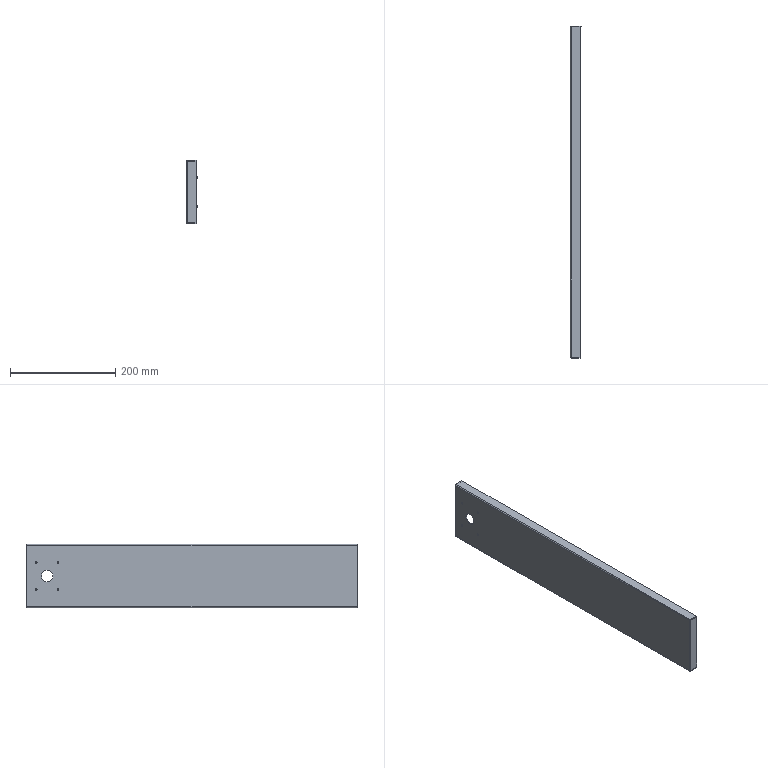Part | STEP file | HESS-408-70-15W-W-20-cabinet lower left outer plate | 1 solid | 56 faces | box 21.5 x 631 x 120 mm | volume 150313 mm3 | plane 38 | cylinder 18 | commonest cylinder face diameters 3.2 x12 0.2 x4 22 x2